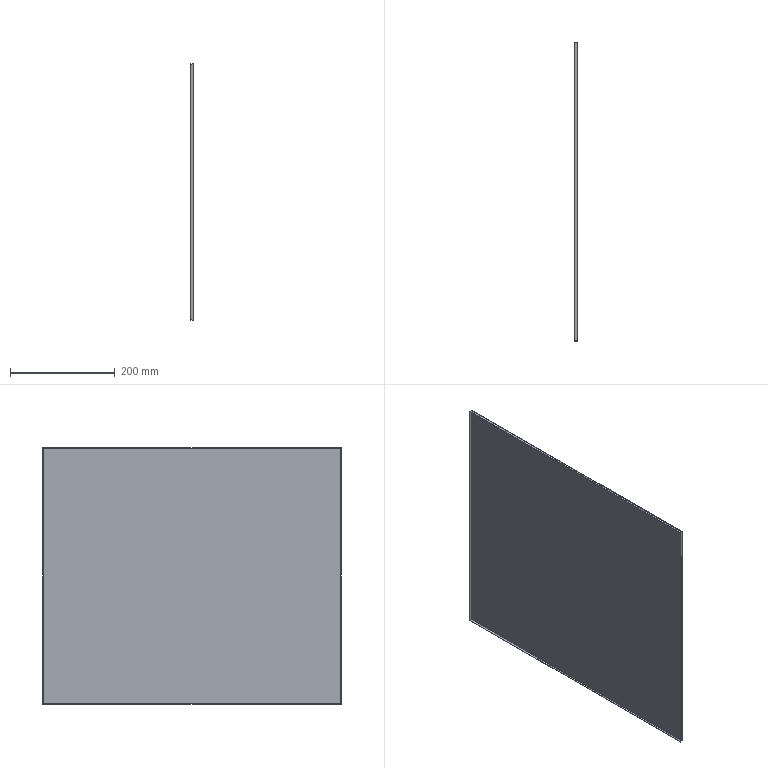Part | STEP file | 01-08 Base frame seal plate 1 | 1 solid | 11 faces | box 5 x 570 x 490 mm | volume 144415 mm3 | plane 11
STEP:
#1=CARTESIAN_POINT('',(0.,0.,0.));
#2=DIRECTION('',(0.,0.,1.));
#3=DIRECTION('',(1.,0.,0.));
#4=AXIS2_PLACEMENT_3D('',#1,#2,#3);
#5=CARTESIAN_POINT('',(-4.5,0.,0.));
#6=VERTEX_POINT('',#5);
#7=CARTESIAN_POINT('',(-4.5,570.,0.));
#8=VERTEX_POINT('',#7);
#9=CARTESIAN_POINT('',(-4.5,285.,0.));
#10=DIRECTION('',(0.,1.,0.));
#11=VECTOR('',#10,1.);
#12=LINE('',#9,#11);
#13=CARTESIAN_POINT('',(0.5,0.,0.));
#14=DIRECTION('',(0.,0.,-1.));
#15=DIRECTION('',(-1.,0.,0.));
#16=AXIS2_PLACEMENT_3D('',#13,#14,#15);
#17=PLANE('',#16);
#18=CARTESIAN_POINT('',(5.,285.));
#19=DIRECTION('',(0.,1.));
#20=VECTOR('',#19,1.);
#21=LINE('',#18,#20);
#22=(GEOMETRIC_REPRESENTATION_CONTEXT(2)PARAMETRIC_REPRESENTATION_CONTEXT()REPRESENTATION_CONTEXT('',''));
#23=DEFINITIONAL_REPRESENTATION('',(#21),#22);
#24=PCURVE('',#17,#23);
#25=CARTESIAN_POINT('',(-4.5,0.,-490.));
#26=DIRECTION('',(-1.,0.,0.));
#27=DIRECTION('',(0.,0.,1.));
#28=AXIS2_PLACEMENT_3D('',#25,#26,#27);
#29=PLANE('',#28);
#30=CARTESIAN_POINT('',(490.,285.));
#31=DIRECTION('',(0.,1.));
#32=VECTOR('',#31,1.);
#33=LINE('',#30,#32);
#34=(GEOMETRIC_REPRESENTATION_CONTEXT(2)PARAMETRIC_REPRESENTATION_CONTEXT()REPRESENTATION_CONTEXT('',''));
#35=DEFINITIONAL_REPRESENTATION('',(#33),#34);
#36=PCURVE('',#29,#35);
#37=SURFACE_CURVE('',#12,(#24,#36),.PCURVE_S1.);
#38=EDGE_CURVE('',#6,#8,#37,.T.);
#39=ORIENTED_EDGE('',*,*,#38,.F.);
#40=CARTESIAN_POINT('',(0.5,0.,0.));
#41=VERTEX_POINT('',#40);
#42=CARTESIAN_POINT('',(-2.,0.,0.));
#43=DIRECTION('',(-1.,0.,0.));
#44=VECTOR('',#43,1.);
#45=LINE('',#42,#44);
#46=CARTESIAN_POINT('',(2.5,0.));
#47=DIRECTION('',(1.,0.));
#48=VECTOR('',#47,1.);
#49=LINE('',#46,#48);
#50=(GEOMETRIC_REPRESENTATION_CONTEXT(2)PARAMETRIC_REPRESENTATION_CONTEXT()REPRESENTATION_CONTEXT('',''));
#51=DEFINITIONAL_REPRESENTATION('',(#49),#50);
#52=PCURVE('',#17,#51);
#53=CARTESIAN_POINT('',(-4.5,0.,-490.));
#54=DIRECTION('',(0.,1.,0.));
#55=DIRECTION('',(0.,0.,1.));
#56=AXIS2_PLACEMENT_3D('',#53,#54,#55);
#57=PLANE('',#56);
#58=CARTESIAN_POINT('',(490.,2.5));
#59=DIRECTION('',(0.,-1.));
#60=VECTOR('',#59,1.);
#61=LINE('',#58,#60);
#62=(GEOMETRIC_REPRESENTATION_CONTEXT(2)PARAMETRIC_REPRESENTATION_CONTEXT()REPRESENTATION_CONTEXT('',''));
#63=DEFINITIONAL_REPRESENTATION('',(#61),#62);
#64=PCURVE('',#57,#63);
#65=SURFACE_CURVE('',#45,(#52,#64),.PCURVE_S1.);
#66=EDGE_CURVE('',#41,#6,#65,.T.);
#67=ORIENTED_EDGE('',*,*,#66,.F.);
#68=CARTESIAN_POINT('',(0.5,570.,0.));
#69=VERTEX_POINT('',#68);
#70=CARTESIAN_POINT('',(0.5,285.,0.));
#71=DIRECTION('',(0.,-1.,0.));
#72=VECTOR('',#71,1.);
#73=LINE('',#70,#72);
#74=CARTESIAN_POINT('',(0.,285.));
#75=DIRECTION('',(0.,-1.));
#76=VECTOR('',#75,1.);
#77=LINE('',#74,#76);
#78=(GEOMETRIC_REPRESENTATION_CONTEXT(2)PARAMETRIC_REPRESENTATION_CONTEXT()REPRESENTATION_CONTEXT('',''));
#79=DEFINITIONAL_REPRESENTATION('',(#77),#78);
#80=PCURVE('',#17,#79);
#81=CARTESIAN_POINT('',(0.5,0.,-490.));
#82=DIRECTION('',(-1.,0.,0.));
#83=DIRECTION('',(0.,0.,1.));
#84=AXIS2_PLACEMENT_3D('',#81,#82,#83);
#85=PLANE('',#84);
#86=CARTESIAN_POINT('',(490.,285.));
#87=DIRECTION('',(0.,-1.));
#88=VECTOR('',#87,1.);
#89=LINE('',#86,#88);
#90=(GEOMETRIC_REPRESENTATION_CONTEXT(2)PARAMETRIC_REPRESENTATION_CONTEXT()REPRESENTATION_CONTEXT('',''));
#91=DEFINITIONAL_REPRESENTATION('',(#89),#90);
#92=PCURVE('',#85,#91);
#93=SURFACE_CURVE('',#73,(#80,#92),.PCURVE_S1.);
#94=EDGE_CURVE('',#69,#41,#93,.T.);
#95=ORIENTED_EDGE('',*,*,#94,.F.);
#96=CARTESIAN_POINT('',(-2.,570.,0.));
#97=DIRECTION('',(1.,0.,0.));
#98=VECTOR('',#97,1.);
#99=LINE('',#96,#98);
#100=CARTESIAN_POINT('',(2.5,570.));
#101=DIRECTION('',(-1.,0.));
#102=VECTOR('',#101,1.);
#103=LINE('',#100,#102);
#104=(GEOMETRIC_REPRESENTATION_CONTEXT(2)PARAMETRIC_REPRESENTATION_CONTEXT()REPRESENTATION_CONTEXT('',''));
#105=DEFINITIONAL_REPRESENTATION('',(#103),#104);
#106=PCURVE('',#17,#105);
#107=CARTESIAN_POINT('',(-4.5,570.,0.));
#108=DIRECTION('',(0.,-1.,0.));
#109=DIRECTION('',(0.,0.,-1.));
#110=AXIS2_PLACEMENT_3D('',#107,#108,#109);
#111=PLANE('',#110);
#112=CARTESIAN_POINT('',(0.,2.5));
#113=DIRECTION('',(0.,1.));
#114=VECTOR('',#113,1.);
#115=LINE('',#112,#114);
#116=(GEOMETRIC_REPRESENTATION_CONTEXT(2)PARAMETRIC_REPRESENTATION_CONTEXT()REPRESENTATION_CONTEXT('',''));
#117=DEFINITIONAL_REPRESENTATION('',(#115),#116);
#118=PCURVE('',#111,#117);
#119=SURFACE_CURVE('',#99,(#106,#118),.PCURVE_S1.);
#120=EDGE_CURVE('',#8,#69,#119,.T.);
#121=ORIENTED_EDGE('',*,*,#120,.F.);
#122=EDGE_LOOP('',(#39,#67,#95,#121));
#123=FACE_BOUND('',#122,.T.);
#124=ADVANCED_FACE('',(#123),#17,.F.);
#125=CARTESIAN_POINT('',(-4.5,570.,-490.));
#126=VERTEX_POINT('',#125);
#127=CARTESIAN_POINT('',(-4.5,570.,-245.));
#128=DIRECTION('',(0.,0.,-1.));
#129=VECTOR('',#128,1.);
#130=LINE('',#127,#129);
#131=CARTESIAN_POINT('',(245.,0.));
#132=DIRECTION('',(1.,0.));
#133=VECTOR('',#132,1.);
#134=LINE('',#131,#133);
#135=(GEOMETRIC_REPRESENTATION_CONTEXT(2)PARAMETRIC_REPRESENTATION_CONTEXT()REPRESENTATION_CONTEXT('',''));
#136=DEFINITIONAL_REPRESENTATION('',(#134),#135);
#137=PCURVE('',#111,#136);
#138=CARTESIAN_POINT('',(245.,570.));
#139=DIRECTION('',(-1.,0.));
#140=VECTOR('',#139,1.);
#141=LINE('',#138,#140);
#142=(GEOMETRIC_REPRESENTATION_CONTEXT(2)PARAMETRIC_REPRESENTATION_CONTEXT()REPRESENTATION_CONTEXT('',''));
#143=DEFINITIONAL_REPRESENTATION('',(#141),#142);
#144=PCURVE('',#29,#143);
#145=SURFACE_CURVE('',#130,(#137,#144),.PCURVE_S1.);
#146=EDGE_CURVE('',#8,#126,#145,.T.);
#147=ORIENTED_EDGE('',*,*,#146,.F.);
#148=ORIENTED_EDGE('',*,*,#120,.T.);
#149=CARTESIAN_POINT('',(0.5,570.,-490.));
#150=VERTEX_POINT('',#149);
#151=CARTESIAN_POINT('',(0.5,570.,-245.));
#152=DIRECTION('',(0.,0.,1.));
#153=VECTOR('',#152,1.);
#154=LINE('',#151,#153);
#155=CARTESIAN_POINT('',(245.,5.));
#156=DIRECTION('',(-1.,0.));
#157=VECTOR('',#156,1.);
#158=LINE('',#155,#157);
#159=(GEOMETRIC_REPRESENTATION_CONTEXT(2)PARAMETRIC_REPRESENTATION_CONTEXT()REPRESENTATION_CONTEXT('',''));
#160=DEFINITIONAL_REPRESENTATION('',(#158),#159);
#161=PCURVE('',#111,#160);
#162=CARTESIAN_POINT('',(245.,570.));
#163=DIRECTION('',(1.,0.));
#164=VECTOR('',#163,1.);
#165=LINE('',#162,#164);
#166=(GEOMETRIC_REPRESENTATION_CONTEXT(2)PARAMETRIC_REPRESENTATION_CONTEXT()REPRESENTATION_CONTEXT('',''));
#167=DEFINITIONAL_REPRESENTATION('',(#165),#166);
#168=PCURVE('',#85,#167);
#169=SURFACE_CURVE('',#154,(#161,#168),.PCURVE_S1.);
#170=EDGE_CURVE('',#150,#69,#169,.T.);
#171=ORIENTED_EDGE('',*,*,#170,.F.);
#172=CARTESIAN_POINT('',(-2.,570.,-490.));
#173=DIRECTION('',(1.,0.,0.));
#174=VECTOR('',#173,1.);
#175=LINE('',#172,#174);
#176=CARTESIAN_POINT('',(490.,2.5));
#177=DIRECTION('',(0.,1.));
#178=VECTOR('',#177,1.);
#179=LINE('',#176,#178);
#180=(GEOMETRIC_REPRESENTATION_CONTEXT(2)PARAMETRIC_REPRESENTATION_CONTEXT()REPRESENTATION_CONTEXT('',''));
#181=DEFINITIONAL_REPRESENTATION('',(#179),#180);
#182=PCURVE('',#111,#181);
#183=CARTESIAN_POINT('',(-4.5,0.,-490.));
#184=DIRECTION('',(0.,0.,1.));
#185=DIRECTION('',(1.,0.,0.));
#186=AXIS2_PLACEMENT_3D('',#183,#184,#185);
#187=PLANE('',#186);
#188=CARTESIAN_POINT('',(2.5,570.));
#189=DIRECTION('',(1.,0.));
#190=VECTOR('',#189,1.);
#191=LINE('',#188,#190);
#192=(GEOMETRIC_REPRESENTATION_CONTEXT(2)PARAMETRIC_REPRESENTATION_CONTEXT()REPRESENTATION_CONTEXT('',''));
#193=DEFINITIONAL_REPRESENTATION('',(#191),#192);
#194=PCURVE('',#187,#193);
#195=SURFACE_CURVE('',#175,(#182,#194),.PCURVE_S1.);
#196=EDGE_CURVE('',#126,#150,#195,.T.);
#197=ORIENTED_EDGE('',*,*,#196,.F.);
#198=EDGE_LOOP('',(#147,#148,#171,#197));
#199=FACE_BOUND('',#198,.T.);
#200=ADVANCED_FACE('',(#199),#111,.F.);
#201=CARTESIAN_POINT('',(-4.5,569.5,-489.5));
#202=VERTEX_POINT('',#201);
#203=CARTESIAN_POINT('',(-4.5,569.5,-0.5));
#204=VERTEX_POINT('',#203);
#205=CARTESIAN_POINT('',(-4.5,569.5,-245.));
#206=DIRECTION('',(0.,0.,1.));
#207=VECTOR('',#206,1.);
#208=LINE('',#205,#207);
#209=CARTESIAN_POINT('',(245.,569.5));
#210=DIRECTION('',(1.,0.));
#211=VECTOR('',#210,1.);
#212=LINE('',#209,#211);
#213=(GEOMETRIC_REPRESENTATION_CONTEXT(2)PARAMETRIC_REPRESENTATION_CONTEXT()REPRESENTATION_CONTEXT('',''));
#214=DEFINITIONAL_REPRESENTATION('',(#212),#213);
#215=PCURVE('',#29,#214);
#216=CARTESIAN_POINT('',(-4.5,569.5,-0.5));
#217=DIRECTION('',(0.,-1.,0.));
#218=DIRECTION('',(0.,0.,-1.));
#219=AXIS2_PLACEMENT_3D('',#216,#217,#218);
#220=PLANE('',#219);
#221=CARTESIAN_POINT('',(244.5,0.));
#222=DIRECTION('',(-1.,0.));
#223=VECTOR('',#222,1.);
#224=LINE('',#221,#223);
#225=(GEOMETRIC_REPRESENTATION_CONTEXT(2)PARAMETRIC_REPRESENTATION_CONTEXT()REPRESENTATION_CONTEXT('',''));
#226=DEFINITIONAL_REPRESENTATION('',(#224),#225);
#227=PCURVE('',#220,#226);
#228=SURFACE_CURVE('',#208,(#215,#227),.PCURVE_S1.);
#229=EDGE_CURVE('',#202,#204,#228,.T.);
#230=ORIENTED_EDGE('',*,*,#229,.T.);
#231=CARTESIAN_POINT('',(-4.5,0.5,-0.5));
#232=VERTEX_POINT('',#231);
#233=CARTESIAN_POINT('',(-4.5,285.,-0.5));
#234=DIRECTION('',(0.,-1.,0.));
#235=VECTOR('',#234,1.);
#236=LINE('',#233,#235);
#237=CARTESIAN_POINT('',(489.5,285.));
#238=DIRECTION('',(0.,-1.));
#239=VECTOR('',#238,1.);
#240=LINE('',#237,#239);
#241=(GEOMETRIC_REPRESENTATION_CONTEXT(2)PARAMETRIC_REPRESENTATION_CONTEXT()REPRESENTATION_CONTEXT('',''));
#242=DEFINITIONAL_REPRESENTATION('',(#240),#241);
#243=PCURVE('',#29,#242);
#244=CARTESIAN_POINT('',(-4.5,0.5,-0.5));
#245=DIRECTION('',(0.,0.,-1.));
#246=DIRECTION('',(0.,1.,0.));
#247=AXIS2_PLACEMENT_3D('',#244,#245,#246);
#248=PLANE('',#247);
#249=CARTESIAN_POINT('',(284.5,0.));
#250=DIRECTION('',(-1.,0.));
#251=VECTOR('',#250,1.);
#252=LINE('',#249,#251);
#253=(GEOMETRIC_REPRESENTATION_CONTEXT(2)PARAMETRIC_REPRESENTATION_CONTEXT()REPRESENTATION_CONTEXT('',''));
#254=DEFINITIONAL_REPRESENTATION('',(#252),#253);
#255=PCURVE('',#248,#254);
#256=SURFACE_CURVE('',#236,(#243,#255),.PCURVE_S1.);
#257=EDGE_CURVE('',#204,#232,#256,.T.);
#258=ORIENTED_EDGE('',*,*,#257,.T.);
#259=CARTESIAN_POINT('',(-4.5,0.5,-489.5));
#260=VERTEX_POINT('',#259);
#261=CARTESIAN_POINT('',(-4.5,0.5,-245.));
#262=DIRECTION('',(0.,0.,-1.));
#263=VECTOR('',#262,1.);
#264=LINE('',#261,#263);
#265=CARTESIAN_POINT('',(245.,0.5));
#266=DIRECTION('',(-1.,0.));
#267=VECTOR('',#266,1.);
#268=LINE('',#265,#267);
#269=(GEOMETRIC_REPRESENTATION_CONTEXT(2)PARAMETRIC_REPRESENTATION_CONTEXT()REPRESENTATION_CONTEXT('',''));
#270=DEFINITIONAL_REPRESENTATION('',(#268),#269);
#271=PCURVE('',#29,#270);
#272=CARTESIAN_POINT('',(-4.5,0.5,-489.5));
#273=DIRECTION('',(0.,1.,0.));
#274=DIRECTION('',(0.,0.,1.));
#275=AXIS2_PLACEMENT_3D('',#272,#273,#274);
#276=PLANE('',#275);
#277=CARTESIAN_POINT('',(244.5,0.));
#278=DIRECTION('',(-1.,0.));
#279=VECTOR('',#278,1.);
#280=LINE('',#277,#279);
#281=(GEOMETRIC_REPRESENTATION_CONTEXT(2)PARAMETRIC_REPRESENTATION_CONTEXT()REPRESENTATION_CONTEXT('',''));
#282=DEFINITIONAL_REPRESENTATION('',(#280),#281);
#283=PCURVE('',#276,#282);
#284=SURFACE_CURVE('',#264,(#271,#283),.PCURVE_S1.);
#285=EDGE_CURVE('',#232,#260,#284,.T.);
#286=ORIENTED_EDGE('',*,*,#285,.T.);
#287=CARTESIAN_POINT('',(-4.5,285.,-489.5));
#288=DIRECTION('',(0.,1.,0.));
#289=VECTOR('',#288,1.);
#290=LINE('',#287,#289);
#291=CARTESIAN_POINT('',(0.5,285.));
#292=DIRECTION('',(0.,1.));
#293=VECTOR('',#292,1.);
#294=LINE('',#291,#293);
#295=(GEOMETRIC_REPRESENTATION_CONTEXT(2)PARAMETRIC_REPRESENTATION_CONTEXT()REPRESENTATION_CONTEXT('',''));
#296=DEFINITIONAL_REPRESENTATION('',(#294),#295);
#297=PCURVE('',#29,#296);
#298=CARTESIAN_POINT('',(-4.5,0.5,-489.5));
#299=DIRECTION('',(0.,0.,1.));
#300=DIRECTION('',(1.,0.,0.));
#301=AXIS2_PLACEMENT_3D('',#298,#299,#300);
#302=PLANE('',#301);
#303=CARTESIAN_POINT('',(0.,284.5));
#304=DIRECTION('',(0.,1.));
#305=VECTOR('',#304,1.);
#306=LINE('',#303,#305);
#307=(GEOMETRIC_REPRESENTATION_CONTEXT(2)PARAMETRIC_REPRESENTATION_CONTEXT()REPRESENTATION_CONTEXT('',''));
#308=DEFINITIONAL_REPRESENTATION('',(#306),#307);
#309=PCURVE('',#302,#308);
#310=SURFACE_CURVE('',#290,(#297,#309),.PCURVE_S1.);
#311=EDGE_CURVE('',#260,#202,#310,.T.);
#312=ORIENTED_EDGE('',*,*,#311,.T.);
#313=EDGE_LOOP('',(#230,#258,#286,#312));
#314=FACE_BOUND('',#313,.T.);
#315=ORIENTED_EDGE('',*,*,#38,.T.);
#316=ORIENTED_EDGE('',*,*,#146,.T.);
#317=CARTESIAN_POINT('',(-4.5,0.,-490.));
#318=VERTEX_POINT('',#317);
#319=CARTESIAN_POINT('',(-4.5,285.,-490.));
#320=DIRECTION('',(0.,-1.,0.));
#321=VECTOR('',#320,1.);
#322=LINE('',#319,#321);
#323=CARTESIAN_POINT('',(0.,285.));
#324=DIRECTION('',(0.,-1.));
#325=VECTOR('',#324,1.);
#326=LINE('',#323,#325);
#327=(GEOMETRIC_REPRESENTATION_CONTEXT(2)PARAMETRIC_REPRESENTATION_CONTEXT()REPRESENTATION_CONTEXT('',''));
#328=DEFINITIONAL_REPRESENTATION('',(#326),#327);
#329=PCURVE('',#29,#328);
#330=CARTESIAN_POINT('',(0.,285.));
#331=DIRECTION('',(0.,-1.));
#332=VECTOR('',#331,1.);
#333=LINE('',#330,#332);
#334=(GEOMETRIC_REPRESENTATION_CONTEXT(2)PARAMETRIC_REPRESENTATION_CONTEXT()REPRESENTATION_CONTEXT('',''));
#335=DEFINITIONAL_REPRESENTATION('',(#333),#334);
#336=PCURVE('',#187,#335);
#337=SURFACE_CURVE('',#322,(#329,#336),.PCURVE_S1.);
#338=EDGE_CURVE('',#126,#318,#337,.T.);
#339=ORIENTED_EDGE('',*,*,#338,.T.);
#340=CARTESIAN_POINT('',(-4.5,0.,-245.));
#341=DIRECTION('',(0.,0.,1.));
#342=VECTOR('',#341,1.);
#343=LINE('',#340,#342);
#344=CARTESIAN_POINT('',(245.,0.));
#345=DIRECTION('',(1.,0.));
#346=VECTOR('',#345,1.);
#347=LINE('',#344,#346);
#348=(GEOMETRIC_REPRESENTATION_CONTEXT(2)PARAMETRIC_REPRESENTATION_CONTEXT()REPRESENTATION_CONTEXT('',''));
#349=DEFINITIONAL_REPRESENTATION('',(#347),#348);
#350=PCURVE('',#29,#349);
#351=CARTESIAN_POINT('',(245.,0.));
#352=DIRECTION('',(1.,0.));
#353=VECTOR('',#352,1.);
#354=LINE('',#351,#353);
#355=(GEOMETRIC_REPRESENTATION_CONTEXT(2)PARAMETRIC_REPRESENTATION_CONTEXT()REPRESENTATION_CONTEXT('',''));
#356=DEFINITIONAL_REPRESENTATION('',(#354),#355);
#357=PCURVE('',#57,#356);
#358=SURFACE_CURVE('',#343,(#350,#357),.PCURVE_S1.);
#359=EDGE_CURVE('',#318,#6,#358,.T.);
#360=ORIENTED_EDGE('',*,*,#359,.T.);
#361=EDGE_LOOP('',(#315,#316,#339,#360));
#362=FACE_BOUND('',#361,.T.);
#363=ADVANCED_FACE('',(#314,#362),#29,.T.);
#364=ORIENTED_EDGE('',*,*,#359,.F.);
#365=CARTESIAN_POINT('',(0.5,0.,-490.));
#366=VERTEX_POINT('',#365);
#367=CARTESIAN_POINT('',(-2.,0.,-490.));
#368=DIRECTION('',(-1.,0.,0.));
#369=VECTOR('',#368,1.);
#370=LINE('',#367,#369);
#371=CARTESIAN_POINT('',(0.,2.5));
#372=DIRECTION('',(0.,-1.));
#373=VECTOR('',#372,1.);
#374=LINE('',#371,#373);
#375=(GEOMETRIC_REPRESENTATION_CONTEXT(2)PARAMETRIC_REPRESENTATION_CONTEXT()REPRESENTATION_CONTEXT('',''));
#376=DEFINITIONAL_REPRESENTATION('',(#374),#375);
#377=PCURVE('',#57,#376);
#378=CARTESIAN_POINT('',(2.5,0.));
#379=DIRECTION('',(-1.,0.));
#380=VECTOR('',#379,1.);
#381=LINE('',#378,#380);
#382=(GEOMETRIC_REPRESENTATION_CONTEXT(2)PARAMETRIC_REPRESENTATION_CONTEXT()REPRESENTATION_CONTEXT('',''));
#383=DEFINITIONAL_REPRESENTATION('',(#381),#382);
#384=PCURVE('',#187,#383);
#385=SURFACE_CURVE('',#370,(#377,#384),.PCURVE_S1.);
#386=EDGE_CURVE('',#366,#318,#385,.T.);
#387=ORIENTED_EDGE('',*,*,#386,.F.);
#388=CARTESIAN_POINT('',(0.5,0.,-245.));
#389=DIRECTION('',(0.,0.,-1.));
#390=VECTOR('',#389,1.);
#391=LINE('',#388,#390);
#392=CARTESIAN_POINT('',(245.,5.));
#393=DIRECTION('',(-1.,0.));
#394=VECTOR('',#393,1.);
#395=LINE('',#392,#394);
#396=(GEOMETRIC_REPRESENTATION_CONTEXT(2)PARAMETRIC_REPRESENTATION_CONTEXT()REPRESENTATION_CONTEXT('',''));
#397=DEFINITIONAL_REPRESENTATION('',(#395),#396);
#398=PCURVE('',#57,#397);
#399=CARTESIAN_POINT('',(245.,0.));
#400=DIRECTION('',(-1.,0.));
#401=VECTOR('',#400,1.);
#402=LINE('',#399,#401);
#403=(GEOMETRIC_REPRESENTATION_CONTEXT(2)PARAMETRIC_REPRESENTATION_CONTEXT()REPRESENTATION_CONTEXT('',''));
#404=DEFINITIONAL_REPRESENTATION('',(#402),#403);
#405=PCURVE('',#85,#404);
#406=SURFACE_CURVE('',#391,(#398,#405),.PCURVE_S1.);
#407=EDGE_CURVE('',#41,#366,#406,.T.);
#408=ORIENTED_EDGE('',*,*,#407,.F.);
#409=ORIENTED_EDGE('',*,*,#66,.T.);
#410=EDGE_LOOP('',(#364,#387,#408,#409));
#411=FACE_BOUND('',#410,.T.);
#412=ADVANCED_FACE('',(#411),#57,.F.);
#413=ORIENTED_EDGE('',*,*,#407,.T.);
#414=CARTESIAN_POINT('',(0.5,285.,-490.));
#415=DIRECTION('',(0.,-1.,0.));
#416=VECTOR('',#415,1.);
#417=LINE('',#414,#416);
#418=CARTESIAN_POINT('',(0.,285.));
#419=DIRECTION('',(0.,-1.));
#420=VECTOR('',#419,1.);
#421=LINE('',#418,#420);
#422=(GEOMETRIC_REPRESENTATION_CONTEXT(2)PARAMETRIC_REPRESENTATION_CONTEXT()REPRESENTATION_CONTEXT('',''));
#423=DEFINITIONAL_REPRESENTATION('',(#421),#422);
#424=PCURVE('',#85,#423);
#425=CARTESIAN_POINT('',(5.,285.));
#426=DIRECTION('',(0.,-1.));
#427=VECTOR('',#426,1.);
#428=LINE('',#425,#427);
#429=(GEOMETRIC_REPRESENTATION_CONTEXT(2)PARAMETRIC_REPRESENTATION_CONTEXT()REPRESENTATION_CONTEXT('',''));
#430=DEFINITIONAL_REPRESENTATION('',(#428),#429);
#431=PCURVE('',#187,#430);
#432=SURFACE_CURVE('',#417,(#424,#431),.PCURVE_S1.);
#433=EDGE_CURVE('',#150,#366,#432,.T.);
#434=ORIENTED_EDGE('',*,*,#433,.F.);
#435=ORIENTED_EDGE('',*,*,#170,.T.);
#436=ORIENTED_EDGE('',*,*,#94,.T.);
#437=EDGE_LOOP('',(#413,#434,#435,#436));
#438=FACE_BOUND('',#437,.T.);
#439=ADVANCED_FACE('',(#438),#85,.F.);
#440=ORIENTED_EDGE('',*,*,#338,.F.);
#441=ORIENTED_EDGE('',*,*,#196,.T.);
#442=ORIENTED_EDGE('',*,*,#433,.T.);
#443=ORIENTED_EDGE('',*,*,#386,.T.);
#444=EDGE_LOOP('',(#440,#441,#442,#443));
#445=FACE_BOUND('',#444,.T.);
#446=ADVANCED_FACE('',(#445),#187,.F.);
#447=ORIENTED_EDGE('',*,*,#257,.F.);
#448=CARTESIAN_POINT('',(0.,569.5,-0.5));
#449=VERTEX_POINT('',#448);
#450=CARTESIAN_POINT('',(-2.25,569.5,-0.5));
#451=DIRECTION('',(1.,0.,0.));
#452=VECTOR('',#451,1.);
#453=LINE('',#450,#452);
#454=CARTESIAN_POINT('',(569.,2.25));
#455=DIRECTION('',(0.,1.));
#456=VECTOR('',#455,1.);
#457=LINE('',#454,#456);
#458=(GEOMETRIC_REPRESENTATION_CONTEXT(2)PARAMETRIC_REPRESENTATION_CONTEXT()REPRESENTATION_CONTEXT('',''));
#459=DEFINITIONAL_REPRESENTATION('',(#457),#458);
#460=PCURVE('',#248,#459);
#461=CARTESIAN_POINT('',(0.,2.25));
#462=DIRECTION('',(0.,1.));
#463=VECTOR('',#462,1.);
#464=LINE('',#461,#463);
#465=(GEOMETRIC_REPRESENTATION_CONTEXT(2)PARAMETRIC_REPRESENTATION_CONTEXT()REPRESENTATION_CONTEXT('',''));
#466=DEFINITIONAL_REPRESENTATION('',(#464),#465);
#467=PCURVE('',#220,#466);
#468=SURFACE_CURVE('',#453,(#460,#467),.PCURVE_S1.);
#469=EDGE_CURVE('',#204,#449,#468,.T.);
#470=ORIENTED_EDGE('',*,*,#469,.T.);
#471=CARTESIAN_POINT('',(0.,0.5,-0.5));
#472=VERTEX_POINT('',#471);
#473=CARTESIAN_POINT('',(0.,285.,-0.5));
#474=DIRECTION('',(0.,-1.,0.));
#475=VECTOR('',#474,1.);
#476=LINE('',#473,#475);
#477=CARTESIAN_POINT('',(284.5,4.5));
#478=DIRECTION('',(-1.,0.));
#479=VECTOR('',#478,1.);
#480=LINE('',#477,#479);
#481=(GEOMETRIC_REPRESENTATION_CONTEXT(2)PARAMETRIC_REPRESENTATION_CONTEXT()REPRESENTATION_CONTEXT('',''));
#482=DEFINITIONAL_REPRESENTATION('',(#480),#481);
#483=PCURVE('',#248,#482);
#484=CARTESIAN_POINT('',(0.,0.5,-489.5));
#485=DIRECTION('',(-1.,0.,0.));
#486=DIRECTION('',(0.,0.,1.));
#487=AXIS2_PLACEMENT_3D('',#484,#485,#486);
#488=PLANE('',#487);
#489=CARTESIAN_POINT('',(489.,284.5));
#490=DIRECTION('',(0.,-1.));
#491=VECTOR('',#490,1.);
#492=LINE('',#489,#491);
#493=(GEOMETRIC_REPRESENTATION_CONTEXT(2)PARAMETRIC_REPRESENTATION_CONTEXT()REPRESENTATION_CONTEXT('',''));
#494=DEFINITIONAL_REPRESENTATION('',(#492),#493);
#495=PCURVE('',#488,#494);
#496=SURFACE_CURVE('',#476,(#483,#495),.PCURVE_S1.);
#497=EDGE_CURVE('',#449,#472,#496,.T.);
#498=ORIENTED_EDGE('',*,*,#497,.T.);
#499=CARTESIAN_POINT('',(-2.25,0.5,-0.5));
#500=DIRECTION('',(-1.,0.,0.));
#501=VECTOR('',#500,1.);
#502=LINE('',#499,#501);
#503=CARTESIAN_POINT('',(0.,2.25));
#504=DIRECTION('',(0.,-1.));
#505=VECTOR('',#504,1.);
#506=LINE('',#503,#505);
#507=(GEOMETRIC_REPRESENTATION_CONTEXT(2)PARAMETRIC_REPRESENTATION_CONTEXT()REPRESENTATION_CONTEXT('',''));
#508=DEFINITIONAL_REPRESENTATION('',(#506),#507);
#509=PCURVE('',#248,#508);
#510=CARTESIAN_POINT('',(489.,2.25));
#511=DIRECTION('',(0.,-1.));
#512=VECTOR('',#511,1.);
#513=LINE('',#510,#512);
#514=(GEOMETRIC_REPRESENTATION_CONTEXT(2)PARAMETRIC_REPRESENTATION_CONTEXT()REPRESENTATION_CONTEXT('',''));
#515=DEFINITIONAL_REPRESENTATION('',(#513),#514);
#516=PCURVE('',#276,#515);
#517=SURFACE_CURVE('',#502,(#509,#516),.PCURVE_S1.);
#518=EDGE_CURVE('',#472,#232,#517,.T.);
#519=ORIENTED_EDGE('',*,*,#518,.T.);
#520=EDGE_LOOP('',(#447,#470,#498,#519));
#521=FACE_BOUND('',#520,.T.);
#522=ADVANCED_FACE('',(#521),#248,.T.);
#523=ORIENTED_EDGE('',*,*,#229,.F.);
#524=CARTESIAN_POINT('',(0.,569.5,-489.5));
#525=VERTEX_POINT('',#524);
#526=CARTESIAN_POINT('',(-2.25,569.5,-489.5));
#527=DIRECTION('',(1.,0.,0.));
#528=VECTOR('',#527,1.);
#529=LINE('',#526,#528);
#530=CARTESIAN_POINT('',(489.,2.25));
#531=DIRECTION('',(0.,1.));
#532=VECTOR('',#531,1.);
#533=LINE('',#530,#532);
#534=(GEOMETRIC_REPRESENTATION_CONTEXT(2)PARAMETRIC_REPRESENTATION_CONTEXT()REPRESENTATION_CONTEXT('',''));
#535=DEFINITIONAL_REPRESENTATION('',(#533),#534);
#536=PCURVE('',#220,#535);
#537=CARTESIAN_POINT('',(2.25,569.));
#538=DIRECTION('',(1.,0.));
#539=VECTOR('',#538,1.);
#540=LINE('',#537,#539);
#541=(GEOMETRIC_REPRESENTATION_CONTEXT(2)PARAMETRIC_REPRESENTATION_CONTEXT()REPRESENTATION_CONTEXT('',''));
#542=DEFINITIONAL_REPRESENTATION('',(#540),#541);
#543=PCURVE('',#302,#542);
#544=SURFACE_CURVE('',#529,(#536,#543),.PCURVE_S1.);
#545=EDGE_CURVE('',#202,#525,#544,.T.);
#546=ORIENTED_EDGE('',*,*,#545,.T.);
#547=CARTESIAN_POINT('',(0.,569.5,-245.));
#548=DIRECTION('',(0.,0.,1.));
#549=VECTOR('',#548,1.);
#550=LINE('',#547,#549);
#551=CARTESIAN_POINT('',(244.5,4.5));
#552=DIRECTION('',(-1.,0.));
#553=VECTOR('',#552,1.);
#554=LINE('',#551,#553);
#555=(GEOMETRIC_REPRESENTATION_CONTEXT(2)PARAMETRIC_REPRESENTATION_CONTEXT()REPRESENTATION_CONTEXT('',''));
#556=DEFINITIONAL_REPRESENTATION('',(#554),#555);
#557=PCURVE('',#220,#556);
#558=CARTESIAN_POINT('',(244.5,569.));
#559=DIRECTION('',(1.,0.));
#560=VECTOR('',#559,1.);
#561=LINE('',#558,#560);
#562=(GEOMETRIC_REPRESENTATION_CONTEXT(2)PARAMETRIC_REPRESENTATION_CONTEXT()REPRESENTATION_CONTEXT('',''));
#563=DEFINITIONAL_REPRESENTATION('',(#561),#562);
#564=PCURVE('',#488,#563);
#565=SURFACE_CURVE('',#550,(#557,#564),.PCURVE_S1.);
#566=EDGE_CURVE('',#525,#449,#565,.T.);
#567=ORIENTED_EDGE('',*,*,#566,.T.);
#568=ORIENTED_EDGE('',*,*,#469,.F.);
#569=EDGE_LOOP('',(#523,#546,#567,#568));
#570=FACE_BOUND('',#569,.T.);
#571=ADVANCED_FACE('',(#570),#220,.T.);
#572=ORIENTED_EDGE('',*,*,#311,.F.);
#573=CARTESIAN_POINT('',(0.,0.5,-489.5));
#574=VERTEX_POINT('',#573);
#575=CARTESIAN_POINT('',(-2.25,0.5,-489.5));
#576=DIRECTION('',(1.,0.,0.));
#577=VECTOR('',#576,1.);
#578=LINE('',#575,#577);
#579=CARTESIAN_POINT('',(2.25,0.));
#580=DIRECTION('',(1.,0.));
#581=VECTOR('',#580,1.);
#582=LINE('',#579,#581);
#583=(GEOMETRIC_REPRESENTATION_CONTEXT(2)PARAMETRIC_REPRESENTATION_CONTEXT()REPRESENTATION_CONTEXT('',''));
#584=DEFINITIONAL_REPRESENTATION('',(#582),#583);
#585=PCURVE('',#302,#584);
#586=CARTESIAN_POINT('',(0.,2.25));
#587=DIRECTION('',(0.,1.));
#588=VECTOR('',#587,1.);
#589=LINE('',#586,#588);
#590=(GEOMETRIC_REPRESENTATION_CONTEXT(2)PARAMETRIC_REPRESENTATION_CONTEXT()REPRESENTATION_CONTEXT('',''));
#591=DEFINITIONAL_REPRESENTATION('',(#589),#590);
#592=PCURVE('',#276,#591);
#593=SURFACE_CURVE('',#578,(#585,#592),.PCURVE_S1.);
#594=EDGE_CURVE('',#260,#574,#593,.T.);
#595=ORIENTED_EDGE('',*,*,#594,.T.);
#596=CARTESIAN_POINT('',(0.,285.,-489.5));
#597=DIRECTION('',(0.,1.,0.));
#598=VECTOR('',#597,1.);
#599=LINE('',#596,#598);
#600=CARTESIAN_POINT('',(4.5,284.5));
#601=DIRECTION('',(0.,1.));
#602=VECTOR('',#601,1.);
#603=LINE('',#600,#602);
#604=(GEOMETRIC_REPRESENTATION_CONTEXT(2)PARAMETRIC_REPRESENTATION_CONTEXT()REPRESENTATION_CONTEXT('',''));
#605=DEFINITIONAL_REPRESENTATION('',(#603),#604);
#606=PCURVE('',#302,#605);
#607=CARTESIAN_POINT('',(0.,284.5));
#608=DIRECTION('',(0.,1.));
#609=VECTOR('',#608,1.);
#610=LINE('',#607,#609);
#611=(GEOMETRIC_REPRESENTATION_CONTEXT(2)PARAMETRIC_REPRESENTATION_CONTEXT()REPRESENTATION_CONTEXT('',''));
#612=DEFINITIONAL_REPRESENTATION('',(#610),#611);
#613=PCURVE('',#488,#612);
#614=SURFACE_CURVE('',#599,(#606,#613),.PCURVE_S1.);
#615=EDGE_CURVE('',#574,#525,#614,.T.);
#616=ORIENTED_EDGE('',*,*,#615,.T.);
#617=ORIENTED_EDGE('',*,*,#545,.F.);
#618=EDGE_LOOP('',(#572,#595,#616,#617));
#619=FACE_BOUND('',#618,.T.);
#620=ADVANCED_FACE('',(#619),#302,.T.);
#621=ORIENTED_EDGE('',*,*,#285,.F.);
#622=ORIENTED_EDGE('',*,*,#518,.F.);
#623=CARTESIAN_POINT('',(0.,0.5,-245.));
#624=DIRECTION('',(0.,0.,-1.));
#625=VECTOR('',#624,1.);
#626=LINE('',#623,#625);
#627=CARTESIAN_POINT('',(244.5,4.5));
#628=DIRECTION('',(-1.,0.));
#629=VECTOR('',#628,1.);
#630=LINE('',#627,#629);
#631=(GEOMETRIC_REPRESENTATION_CONTEXT(2)PARAMETRIC_REPRESENTATION_CONTEXT()REPRESENTATION_CONTEXT('',''));
#632=DEFINITIONAL_REPRESENTATION('',(#630),#631);
#633=PCURVE('',#276,#632);
#634=CARTESIAN_POINT('',(244.5,0.));
#635=DIRECTION('',(-1.,0.));
#636=VECTOR('',#635,1.);
#637=LINE('',#634,#636);
#638=(GEOMETRIC_REPRESENTATION_CONTEXT(2)PARAMETRIC_REPRESENTATION_CONTEXT()REPRESENTATION_CONTEXT('',''));
#639=DEFINITIONAL_REPRESENTATION('',(#637),#638);
#640=PCURVE('',#488,#639);
#641=SURFACE_CURVE('',#626,(#633,#640),.PCURVE_S1.);
#642=EDGE_CURVE('',#472,#574,#641,.T.);
#643=ORIENTED_EDGE('',*,*,#642,.T.);
#644=ORIENTED_EDGE('',*,*,#594,.F.);
#645=EDGE_LOOP('',(#621,#622,#643,#644));
#646=FACE_BOUND('',#645,.T.);
#647=ADVANCED_FACE('',(#646),#276,.T.);
#648=ORIENTED_EDGE('',*,*,#497,.F.);
#649=ORIENTED_EDGE('',*,*,#566,.F.);
#650=ORIENTED_EDGE('',*,*,#615,.F.);
#651=ORIENTED_EDGE('',*,*,#642,.F.);
#652=EDGE_LOOP('',(#648,#649,#650,#651));
#653=FACE_BOUND('',#652,.T.);
#654=ADVANCED_FACE('',(#653),#488,.T.);
#655=CLOSED_SHELL('',(#124,#200,#363,#412,#439,#446,#522,#571,#620,#647,#654));
#656=MANIFOLD_SOLID_BREP('',#655);
#657=(LENGTH_UNIT()NAMED_UNIT(*)SI_UNIT(.MILLI.,.METRE.));
#658=UNCERTAINTY_MEASURE_WITH_UNIT(LENGTH_MEASURE(0.0000001),#657,'','');
#659=(NAMED_UNIT(*)PLANE_ANGLE_UNIT()SI_UNIT($,.RADIAN.));
#660=(NAMED_UNIT(*)SI_UNIT($,.STERADIAN.)SOLID_ANGLE_UNIT());
#661=(GEOMETRIC_REPRESENTATION_CONTEXT(3)GLOBAL_UNCERTAINTY_ASSIGNED_CONTEXT((#658))GLOBAL_UNIT_ASSIGNED_CONTEXT((#657,#659,#660))REPRESENTATION_CONTEXT('',''));
#662=ADVANCED_BREP_SHAPE_REPRESENTATION('',(#4,#656),#661);